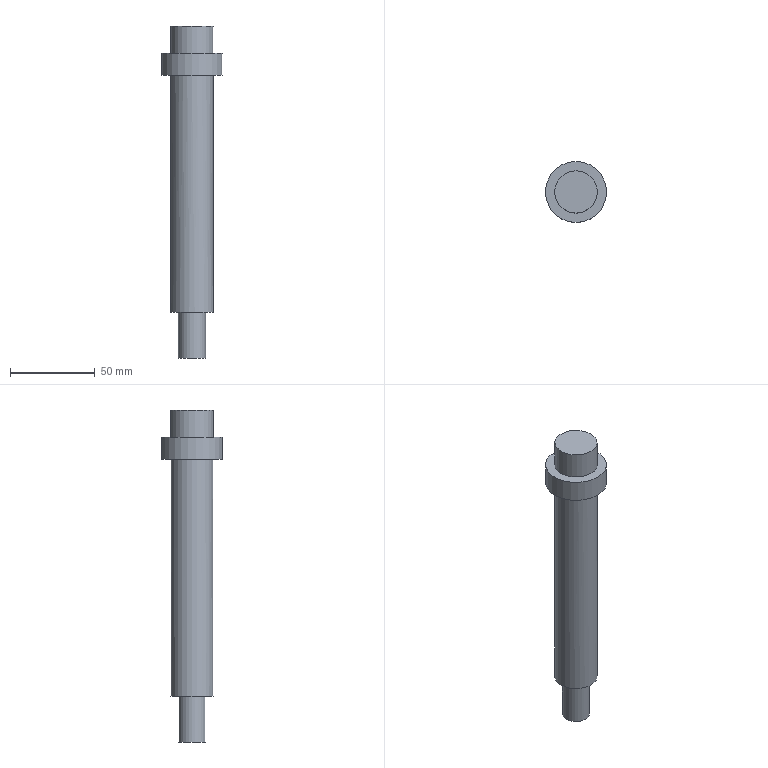Part | NX | features solid 2 | 1 solid | 9 faces | box 36 x 36 x 196 mm | volume 95237 mm3 | plane 5 | cylinder 4 | commonest cylinder face diameters 25 x2 16 x1 36 x1
STEP:
#1=CARTESIAN_POINT('',(47.,-280.,50.));
#2=VERTEX_POINT('',#1);
#3=CARTESIAN_POINT('',(55.,-280.,50.));
#4=DIRECTION('',(0.,0.,-1.));
#5=DIRECTION('',(-1.,0.,0.));
#6=AXIS2_PLACEMENT_3D('',#3,#4,#5);
#7=CIRCLE('',#6,8.);
#8=EDGE_CURVE('',#2,#2,#7,.F.);
#9=ORIENTED_EDGE('',*,*,#8,.T.);
#10=EDGE_LOOP('',(#9));
#11=FACE_BOUND('',#10,.T.);
#12=CARTESIAN_POINT('',(42.5,-280.,50.));
#13=VERTEX_POINT('',#12);
#14=CARTESIAN_POINT('',(55.,-280.,50.));
#15=DIRECTION('',(0.,0.,-1.));
#16=DIRECTION('',(-1.,0.,0.));
#17=AXIS2_PLACEMENT_3D('',#14,#15,#16);
#18=CIRCLE('',#17,12.5);
#19=EDGE_CURVE('',#13,#13,#18,.T.);
#20=ORIENTED_EDGE('',*,*,#19,.T.);
#21=EDGE_LOOP('',(#20));
#22=FACE_BOUND('',#21,.T.);
#23=CARTESIAN_POINT('',(55.,-280.,50.));
#24=DIRECTION('',(0.,0.,-1.));
#25=DIRECTION('',(0.,-1.,0.));
#26=AXIS2_PLACEMENT_3D('',#23,#24,#25);
#27=PLANE('',#26);
#28=ADVANCED_FACE('',(#11,#22),#27,.T.);
#29=CARTESIAN_POINT('',(55.,-292.5,190.));
#30=VERTEX_POINT('',#29);
#31=CARTESIAN_POINT('',(55.,-280.,190.));
#32=DIRECTION('',(0.,0.,1.));
#33=DIRECTION('',(0.,-1.,0.));
#34=AXIS2_PLACEMENT_3D('',#31,#32,#33);
#35=CIRCLE('',#34,12.5);
#36=EDGE_CURVE('',#30,#30,#35,.F.);
#37=ORIENTED_EDGE('',*,*,#36,.T.);
#38=EDGE_LOOP('',(#37));
#39=FACE_BOUND('',#38,.T.);
#40=ORIENTED_EDGE('',*,*,#19,.F.);
#41=EDGE_LOOP('',(#40));
#42=FACE_BOUND('',#41,.T.);
#43=CARTESIAN_POINT('',(55.,-280.,-50.));
#44=DIRECTION('',(0.,0.,1.));
#45=DIRECTION('',(0.,1.,0.));
#46=AXIS2_PLACEMENT_3D('',#43,#44,#45);
#47=CYLINDRICAL_SURFACE('',#46,12.5);
#48=ADVANCED_FACE('',(#39,#42),#47,.T.);
#49=CARTESIAN_POINT('',(47.,-280.,23.));
#50=VERTEX_POINT('',#49);
#51=CARTESIAN_POINT('',(55.,-280.,23.));
#52=DIRECTION('',(0.,0.,-1.));
#53=DIRECTION('',(-1.,0.,0.));
#54=AXIS2_PLACEMENT_3D('',#51,#52,#53);
#55=CIRCLE('',#54,8.);
#56=EDGE_CURVE('',#50,#50,#55,.T.);
#57=ORIENTED_EDGE('',*,*,#56,.T.);
#58=EDGE_LOOP('',(#57));
#59=FACE_BOUND('',#58,.T.);
#60=CARTESIAN_POINT('',(55.,-280.,23.));
#61=DIRECTION('',(0.,0.,-1.));
#62=DIRECTION('',(0.,-1.,0.));
#63=AXIS2_PLACEMENT_3D('',#60,#61,#62);
#64=PLANE('',#63);
#65=ADVANCED_FACE('',(#59),#64,.T.);
#66=ORIENTED_EDGE('',*,*,#56,.F.);
#67=EDGE_LOOP('',(#66));
#68=FACE_BOUND('',#67,.T.);
#69=ORIENTED_EDGE('',*,*,#8,.F.);
#70=EDGE_LOOP('',(#69));
#71=FACE_BOUND('',#70,.T.);
#72=CARTESIAN_POINT('',(55.,-280.,-50.));
#73=DIRECTION('',(0.,0.,-1.));
#74=DIRECTION('',(0.,-1.,0.));
#75=AXIS2_PLACEMENT_3D('',#72,#73,#74);
#76=CYLINDRICAL_SURFACE('',#75,8.);
#77=ADVANCED_FACE('',(#68,#71),#76,.T.);
#78=CARTESIAN_POINT('',(55.,-267.5,203.));
#79=VERTEX_POINT('',#78);
#80=CARTESIAN_POINT('',(55.,-280.,203.));
#81=DIRECTION('',(0.,0.,-1.));
#82=DIRECTION('',(0.,1.,0.));
#83=AXIS2_PLACEMENT_3D('',#80,#81,#82);
#84=CIRCLE('',#83,12.5);
#85=EDGE_CURVE('',#79,#79,#84,.T.);
#86=ORIENTED_EDGE('',*,*,#85,.T.);
#87=EDGE_LOOP('',(#86));
#88=FACE_BOUND('',#87,.T.);
#89=CARTESIAN_POINT('',(55.,-298.,203.));
#90=VERTEX_POINT('',#89);
#91=CARTESIAN_POINT('',(55.,-280.,203.));
#92=DIRECTION('',(0.,0.,1.));
#93=DIRECTION('',(0.,-1.,0.));
#94=AXIS2_PLACEMENT_3D('',#91,#92,#93);
#95=CIRCLE('',#94,18.);
#96=EDGE_CURVE('',#90,#90,#95,.T.);
#97=ORIENTED_EDGE('',*,*,#96,.T.);
#98=EDGE_LOOP('',(#97));
#99=FACE_BOUND('',#98,.T.);
#100=CARTESIAN_POINT('',(55.,-280.,203.));
#101=DIRECTION('',(0.,0.,1.));
#102=DIRECTION('',(0.,1.,0.));
#103=AXIS2_PLACEMENT_3D('',#100,#101,#102);
#104=PLANE('',#103);
#105=ADVANCED_FACE('',(#88,#99),#104,.T.);
#106=ORIENTED_EDGE('',*,*,#36,.F.);
#107=EDGE_LOOP('',(#106));
#108=FACE_BOUND('',#107,.T.);
#109=CARTESIAN_POINT('',(55.,-262.,190.));
#110=VERTEX_POINT('',#109);
#111=CARTESIAN_POINT('',(55.,-280.,190.));
#112=DIRECTION('',(0.,0.,-1.));
#113=DIRECTION('',(0.,1.,0.));
#114=AXIS2_PLACEMENT_3D('',#111,#112,#113);
#115=CIRCLE('',#114,18.);
#116=EDGE_CURVE('',#110,#110,#115,.T.);
#117=ORIENTED_EDGE('',*,*,#116,.T.);
#118=EDGE_LOOP('',(#117));
#119=FACE_BOUND('',#118,.T.);
#120=CARTESIAN_POINT('',(55.,-280.,190.));
#121=DIRECTION('',(0.,0.,-1.));
#122=DIRECTION('',(0.,-1.,0.));
#123=AXIS2_PLACEMENT_3D('',#120,#121,#122);
#124=PLANE('',#123);
#125=ADVANCED_FACE('',(#108,#119),#124,.T.);
#126=ORIENTED_EDGE('',*,*,#96,.F.);
#127=EDGE_LOOP('',(#126));
#128=FACE_BOUND('',#127,.T.);
#129=ORIENTED_EDGE('',*,*,#116,.F.);
#130=EDGE_LOOP('',(#129));
#131=FACE_BOUND('',#130,.T.);
#132=CARTESIAN_POINT('',(55.,-280.,190.));
#133=DIRECTION('',(0.,0.,1.));
#134=DIRECTION('',(0.,1.,0.));
#135=AXIS2_PLACEMENT_3D('',#132,#133,#134);
#136=CYLINDRICAL_SURFACE('',#135,18.);
#137=ADVANCED_FACE('',(#128,#131),#136,.T.);
#138=CARTESIAN_POINT('',(55.,-292.5,219.));
#139=VERTEX_POINT('',#138);
#140=CARTESIAN_POINT('',(55.,-280.,219.));
#141=DIRECTION('',(0.,0.,1.));
#142=DIRECTION('',(0.,-1.,0.));
#143=AXIS2_PLACEMENT_3D('',#140,#141,#142);
#144=CIRCLE('',#143,12.5);
#145=EDGE_CURVE('',#139,#139,#144,.T.);
#146=ORIENTED_EDGE('',*,*,#145,.T.);
#147=EDGE_LOOP('',(#146));
#148=FACE_BOUND('',#147,.T.);
#149=CARTESIAN_POINT('',(55.,-280.,219.));
#150=DIRECTION('',(0.,0.,1.));
#151=DIRECTION('',(0.,1.,0.));
#152=AXIS2_PLACEMENT_3D('',#149,#150,#151);
#153=PLANE('',#152);
#154=ADVANCED_FACE('',(#148),#153,.T.);
#155=ORIENTED_EDGE('',*,*,#145,.F.);
#156=EDGE_LOOP('',(#155));
#157=FACE_BOUND('',#156,.T.);
#158=ORIENTED_EDGE('',*,*,#85,.F.);
#159=EDGE_LOOP('',(#158));
#160=FACE_BOUND('',#159,.T.);
#161=CARTESIAN_POINT('',(55.,-280.,203.));
#162=DIRECTION('',(0.,0.,1.));
#163=DIRECTION('',(0.,1.,0.));
#164=AXIS2_PLACEMENT_3D('',#161,#162,#163);
#165=CYLINDRICAL_SURFACE('',#164,12.5);
#166=ADVANCED_FACE('',(#157,#160),#165,.T.);
#167=CLOSED_SHELL('',(#28,#48,#65,#77,#105,#125,#137,#154,#166));
#168=MANIFOLD_SOLID_BREP('',#167);
#169=(LENGTH_UNIT()NAMED_UNIT(*)SI_UNIT(.MILLI.,.METRE.));
#170=UNCERTAINTY_MEASURE_WITH_UNIT(LENGTH_MEASURE(0.00001),#169,'','');
#171=(NAMED_UNIT(*)PLANE_ANGLE_UNIT()SI_UNIT($,.RADIAN.));
#172=(NAMED_UNIT(*)SI_UNIT($,.STERADIAN.)SOLID_ANGLE_UNIT());
#173=(GEOMETRIC_REPRESENTATION_CONTEXT(3)GLOBAL_UNCERTAINTY_ASSIGNED_CONTEXT((#170))GLOBAL_UNIT_ASSIGNED_CONTEXT((#169,#171,#172))REPRESENTATION_CONTEXT('',''));
#174=ADVANCED_BREP_SHAPE_REPRESENTATION('',(#168),#173);